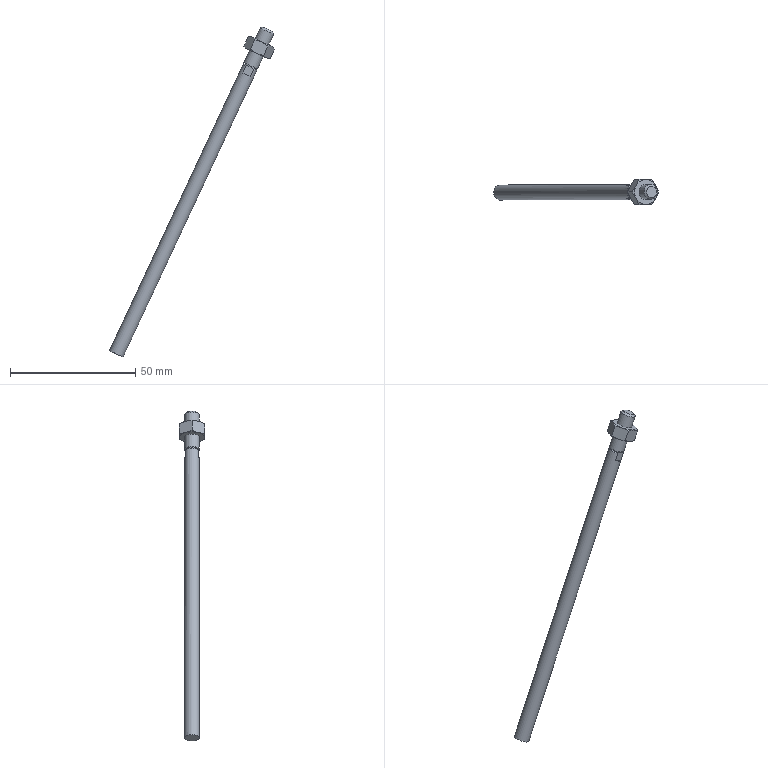Part | STEP file | 冲床-300配套压波_id674_x_t | 1 solid | 36 faces | box 65.907 x 10 x 131.805 mm | volume 4315 mm3 | plane 17 | cone 15 | cylinder 4 | commonest cylinder face diameters 6 x3 5 x1
STEP:
#1=CARTESIAN_POINT('',(2039.756,5.,-415.059));
#2=VERTEX_POINT('',#1);
#3=CARTESIAN_POINT('',(2036.951,5.,-414.243));
#4=VERTEX_POINT('',#3);
#5=CARTESIAN_POINT('',(2039.756,5.,-415.059));
#6=CARTESIAN_POINT('',(2038.786,5.,-414.907));
#7=CARTESIAN_POINT('',(2037.844,5.,-414.66));
#8=CARTESIAN_POINT('',(2036.951,5.,-414.243));
#9=B_SPLINE_CURVE_WITH_KNOTS('',3,(#5,#6,#7,#8),.UNSPECIFIED.,.F.,.F.,(4,4),(0.,1.),.UNSPECIFIED.);
#10=EDGE_CURVE('',#2,#4,#9,.T.);
#11=ORIENTED_EDGE('',*,*,#10,.T.);
#12=CARTESIAN_POINT('',(2034.524,5.,-412.618));
#13=VERTEX_POINT('',#12);
#14=CARTESIAN_POINT('',(2036.951,5.,-414.243));
#15=CARTESIAN_POINT('',(2036.058,5.,-413.827));
#16=CARTESIAN_POINT('',(2035.263,5.,-413.264));
#17=CARTESIAN_POINT('',(2034.524,5.,-412.618));
#18=B_SPLINE_CURVE_WITH_KNOTS('',3,(#14,#15,#16,#17),.UNSPECIFIED.,.F.,.F.,(4,4),(0.,1.),.UNSPECIFIED.);
#19=EDGE_CURVE('',#4,#13,#18,.T.);
#20=ORIENTED_EDGE('',*,*,#19,.T.);
#21=CARTESIAN_POINT('',(2036.261,5.,-408.896));
#22=VERTEX_POINT('',#21);
#23=CARTESIAN_POINT('',(2034.335,5.,-413.023));
#24=DIRECTION('',(0.4229,0.,0.9062));
#25=VECTOR('',#24,1.);
#26=LINE('',#23,#25);
#27=EDGE_CURVE('',#13,#22,#26,.T.);
#28=ORIENTED_EDGE('',*,*,#27,.T.);
#29=CARTESIAN_POINT('',(2039.065,5.,-409.712));
#30=VERTEX_POINT('',#29);
#31=CARTESIAN_POINT('',(2036.261,5.,-408.896));
#32=CARTESIAN_POINT('',(2037.23,5.,-409.049));
#33=CARTESIAN_POINT('',(2038.173,5.,-409.296));
#34=CARTESIAN_POINT('',(2039.065,5.,-409.712));
#35=B_SPLINE_CURVE_WITH_KNOTS('',3,(#31,#32,#33,#34),.UNSPECIFIED.,.F.,.F.,(4,4),(0.,1.),.UNSPECIFIED.);
#36=EDGE_CURVE('',#22,#30,#35,.T.);
#37=ORIENTED_EDGE('',*,*,#36,.T.);
#38=CARTESIAN_POINT('',(2041.493,5.,-411.338));
#39=VERTEX_POINT('',#38);
#40=CARTESIAN_POINT('',(2039.065,5.,-409.712));
#41=CARTESIAN_POINT('',(2039.958,5.,-410.129));
#42=CARTESIAN_POINT('',(2040.753,5.,-410.692));
#43=CARTESIAN_POINT('',(2041.493,5.,-411.338));
#44=B_SPLINE_CURVE_WITH_KNOTS('',3,(#40,#41,#42,#43),.UNSPECIFIED.,.F.,.F.,(4,4),(0.,1.),.UNSPECIFIED.);
#45=EDGE_CURVE('',#30,#39,#44,.T.);
#46=ORIENTED_EDGE('',*,*,#45,.T.);
#47=CARTESIAN_POINT('',(2039.567,5.,-415.464));
#48=DIRECTION('',(0.4229,0.,0.9062));
#49=VECTOR('',#48,1.);
#50=LINE('',#47,#49);
#51=EDGE_CURVE('',#2,#39,#50,.T.);
#52=ORIENTED_EDGE('',*,*,#51,.F.);
#53=EDGE_LOOP('',(#11,#20,#28,#37,#46,#52));
#54=FACE_OUTER_BOUND('',#53,.T.);
#55=CARTESIAN_POINT('',(2039.567,5.,-415.464));
#56=DIRECTION('',(0.,1.,0.));
#57=DIRECTION('',(0.9062,0.,-0.4229));
#58=AXIS2_PLACEMENT_3D('',#55,#56,#57);
#59=PLANE('',#58);
#60=ADVANCED_FACE('',(#54),#59,.T.);
#61=CARTESIAN_POINT('',(2042.372,0.,-416.28));
#62=VERTEX_POINT('',#61);
#63=CARTESIAN_POINT('',(2040.875,2.5,-416.074));
#64=VERTEX_POINT('',#63);
#65=CARTESIAN_POINT('',(2042.372,0.,-416.28));
#66=CARTESIAN_POINT('',(2041.829,0.8168,-416.327));
#67=CARTESIAN_POINT('',(2041.321,1.647,-416.283));
#68=CARTESIAN_POINT('',(2040.875,2.5,-416.074));
#69=B_SPLINE_CURVE_WITH_KNOTS('',3,(#65,#66,#67,#68),.UNSPECIFIED.,.F.,.F.,(4,4),(0.,1.),.UNSPECIFIED.);
#70=EDGE_CURVE('',#62,#64,#69,.T.);
#71=ORIENTED_EDGE('',*,*,#70,.T.);
#72=CARTESIAN_POINT('',(2040.875,2.5,-416.074));
#73=CARTESIAN_POINT('',(2040.429,3.353,-415.866));
#74=CARTESIAN_POINT('',(2040.068,4.183,-415.506));
#75=CARTESIAN_POINT('',(2039.756,5.,-415.059));
#76=B_SPLINE_CURVE_WITH_KNOTS('',3,(#72,#73,#74,#75),.UNSPECIFIED.,.F.,.F.,(4,4),(0.,1.),.UNSPECIFIED.);
#77=EDGE_CURVE('',#64,#2,#76,.T.);
#78=ORIENTED_EDGE('',*,*,#77,.T.);
#79=ORIENTED_EDGE('',*,*,#51,.T.);
#80=CARTESIAN_POINT('',(2042.989,2.5,-411.544));
#81=VERTEX_POINT('',#80);
#82=CARTESIAN_POINT('',(2041.493,5.,-411.338));
#83=CARTESIAN_POINT('',(2042.035,4.183,-411.291));
#84=CARTESIAN_POINT('',(2042.543,3.353,-411.335));
#85=CARTESIAN_POINT('',(2042.989,2.5,-411.544));
#86=B_SPLINE_CURVE_WITH_KNOTS('',3,(#82,#83,#84,#85),.UNSPECIFIED.,.F.,.F.,(4,4),(0.,1.),.UNSPECIFIED.);
#87=EDGE_CURVE('',#39,#81,#86,.T.);
#88=ORIENTED_EDGE('',*,*,#87,.T.);
#89=CARTESIAN_POINT('',(2044.108,0.,-412.559));
#90=VERTEX_POINT('',#89);
#91=CARTESIAN_POINT('',(2042.989,2.5,-411.544));
#92=CARTESIAN_POINT('',(2043.436,1.647,-411.752));
#93=CARTESIAN_POINT('',(2043.796,0.8168,-412.112));
#94=CARTESIAN_POINT('',(2044.108,0.,-412.559));
#95=B_SPLINE_CURVE_WITH_KNOTS('',3,(#91,#92,#93,#94),.UNSPECIFIED.,.F.,.F.,(4,4),(0.,1.),.UNSPECIFIED.);
#96=EDGE_CURVE('',#81,#90,#95,.T.);
#97=ORIENTED_EDGE('',*,*,#96,.T.);
#98=CARTESIAN_POINT('',(2042.183,0.,-416.685));
#99=DIRECTION('',(0.4229,0.,0.9062));
#100=VECTOR('',#99,1.);
#101=LINE('',#98,#100);
#102=EDGE_CURVE('',#62,#90,#101,.T.);
#103=ORIENTED_EDGE('',*,*,#102,.F.);
#104=EDGE_LOOP('',(#71,#78,#79,#88,#97,#103));
#105=FACE_OUTER_BOUND('',#104,.T.);
#106=CARTESIAN_POINT('',(2042.183,0.,-416.685));
#107=DIRECTION('',(0.7848,0.5,-0.3662));
#108=DIRECTION('',(0.4531,-0.866,-0.2114));
#109=AXIS2_PLACEMENT_3D('',#106,#107,#108);
#110=PLANE('',#109);
#111=ADVANCED_FACE('',(#105),#110,.T.);
#112=ORIENTED_EDGE('',*,*,#10,.F.);
#113=ORIENTED_EDGE('',*,*,#77,.F.);
#114=CARTESIAN_POINT('',(2036.951,0.,-414.243));
#115=DIRECTION('',(0.4229,0.,0.9062));
#116=DIRECTION('',(0.,-1.,0.));
#117=AXIS2_PLACEMENT_3D('',#114,#115,#116);
#118=CIRCLE('',#117,5.);
#119=EDGE_CURVE('',#64,#4,#118,.T.);
#120=ORIENTED_EDGE('',*,*,#119,.T.);
#121=EDGE_LOOP('',(#112,#113,#120));
#122=FACE_OUTER_BOUND('',#121,.T.);
#123=CARTESIAN_POINT('',(2036.951,0.,-414.243));
#124=DIRECTION('',(0.4229,0.,0.9062));
#125=DIRECTION('',(0.,1.,0.));
#126=AXIS2_PLACEMENT_3D('',#123,#124,#125);
#127=CONICAL_SURFACE('',#126,5.,60.);
#128=ADVANCED_FACE('',(#122),#127,.T.);
#129=ORIENTED_EDGE('',*,*,#45,.F.);
#130=CARTESIAN_POINT('',(2039.065,0.,-409.712));
#131=DIRECTION('',(0.4229,0.,0.9062));
#132=DIRECTION('',(0.,-1.,0.));
#133=AXIS2_PLACEMENT_3D('',#130,#131,#132);
#134=CIRCLE('',#133,5.);
#135=EDGE_CURVE('',#81,#30,#134,.T.);
#136=ORIENTED_EDGE('',*,*,#135,.F.);
#137=ORIENTED_EDGE('',*,*,#87,.F.);
#138=EDGE_LOOP('',(#129,#136,#137));
#139=FACE_OUTER_BOUND('',#138,.T.);
#140=CARTESIAN_POINT('',(2038.877,0.,-410.117));
#141=DIRECTION('',(-0.4229,0.,-0.9062));
#142=DIRECTION('',(0.,-1.,0.));
#143=AXIS2_PLACEMENT_3D('',#140,#141,#142);
#144=CONICAL_SURFACE('',#143,5.774,60.);
#145=ADVANCED_FACE('',(#139),#144,.T.);
#146=CARTESIAN_POINT('',(2033.027,2.5,-412.412));
#147=VERTEX_POINT('',#146);
#148=CARTESIAN_POINT('',(2034.524,5.,-412.618));
#149=CARTESIAN_POINT('',(2033.981,4.183,-412.665));
#150=CARTESIAN_POINT('',(2033.474,3.353,-412.621));
#151=CARTESIAN_POINT('',(2033.027,2.5,-412.412));
#152=B_SPLINE_CURVE_WITH_KNOTS('',3,(#148,#149,#150,#151),.UNSPECIFIED.,.F.,.F.,(4,4),(0.,1.),.UNSPECIFIED.);
#153=EDGE_CURVE('',#13,#147,#152,.T.);
#154=ORIENTED_EDGE('',*,*,#153,.F.);
#155=ORIENTED_EDGE('',*,*,#19,.F.);
#156=CARTESIAN_POINT('',(2036.951,0.,-414.243));
#157=DIRECTION('',(0.4229,0.,0.9062));
#158=DIRECTION('',(0.,-1.,0.));
#159=AXIS2_PLACEMENT_3D('',#156,#157,#158);
#160=CIRCLE('',#159,5.);
#161=EDGE_CURVE('',#4,#147,#160,.T.);
#162=ORIENTED_EDGE('',*,*,#161,.T.);
#163=EDGE_LOOP('',(#154,#155,#162));
#164=FACE_OUTER_BOUND('',#163,.T.);
#165=CARTESIAN_POINT('',(2036.951,0.,-414.243));
#166=DIRECTION('',(0.4229,0.,0.9062));
#167=DIRECTION('',(0.,1.,0.));
#168=AXIS2_PLACEMENT_3D('',#165,#166,#167);
#169=CONICAL_SURFACE('',#168,5.,60.);
#170=ADVANCED_FACE('',(#164),#169,.T.);
#171=CARTESIAN_POINT('',(2035.141,2.5,-407.881));
#172=VERTEX_POINT('',#171);
#173=CARTESIAN_POINT('',(2035.141,2.5,-407.881));
#174=CARTESIAN_POINT('',(2035.588,3.353,-408.09));
#175=CARTESIAN_POINT('',(2035.948,4.183,-408.45));
#176=CARTESIAN_POINT('',(2036.261,5.,-408.896));
#177=B_SPLINE_CURVE_WITH_KNOTS('',3,(#173,#174,#175,#176),.UNSPECIFIED.,.F.,.F.,(4,4),(0.,1.),.UNSPECIFIED.);
#178=EDGE_CURVE('',#172,#22,#177,.T.);
#179=ORIENTED_EDGE('',*,*,#178,.F.);
#180=CARTESIAN_POINT('',(2039.065,0.,-409.712));
#181=DIRECTION('',(0.4229,0.,0.9062));
#182=DIRECTION('',(0.,-1.,0.));
#183=AXIS2_PLACEMENT_3D('',#180,#181,#182);
#184=CIRCLE('',#183,5.);
#185=EDGE_CURVE('',#30,#172,#184,.T.);
#186=ORIENTED_EDGE('',*,*,#185,.F.);
#187=ORIENTED_EDGE('',*,*,#36,.F.);
#188=EDGE_LOOP('',(#179,#186,#187));
#189=FACE_OUTER_BOUND('',#188,.T.);
#190=CARTESIAN_POINT('',(2038.877,0.,-410.117));
#191=DIRECTION('',(-0.4229,0.,-0.9062));
#192=DIRECTION('',(0.,-1.,0.));
#193=AXIS2_PLACEMENT_3D('',#190,#191,#192);
#194=CONICAL_SURFACE('',#193,5.774,60.);
#195=ADVANCED_FACE('',(#189),#194,.T.);
#196=ORIENTED_EDGE('',*,*,#153,.T.);
#197=CARTESIAN_POINT('',(2031.908,0.,-411.397));
#198=VERTEX_POINT('',#197);
#199=CARTESIAN_POINT('',(2033.027,2.5,-412.412));
#200=CARTESIAN_POINT('',(2032.581,1.647,-412.204));
#201=CARTESIAN_POINT('',(2032.22,0.8168,-411.843));
#202=CARTESIAN_POINT('',(2031.908,0.,-411.397));
#203=B_SPLINE_CURVE_WITH_KNOTS('',3,(#199,#200,#201,#202),.UNSPECIFIED.,.F.,.F.,(4,4),(0.,1.),.UNSPECIFIED.);
#204=EDGE_CURVE('',#147,#198,#203,.T.);
#205=ORIENTED_EDGE('',*,*,#204,.T.);
#206=CARTESIAN_POINT('',(2033.645,0.,-407.676));
#207=VERTEX_POINT('',#206);
#208=CARTESIAN_POINT('',(2031.719,0.,-411.802));
#209=DIRECTION('',(0.4229,0.,0.9062));
#210=VECTOR('',#209,1.);
#211=LINE('',#208,#210);
#212=EDGE_CURVE('',#198,#207,#211,.T.);
#213=ORIENTED_EDGE('',*,*,#212,.T.);
#214=CARTESIAN_POINT('',(2033.645,0.,-407.676));
#215=CARTESIAN_POINT('',(2034.187,0.8168,-407.628));
#216=CARTESIAN_POINT('',(2034.695,1.647,-407.673));
#217=CARTESIAN_POINT('',(2035.141,2.5,-407.881));
#218=B_SPLINE_CURVE_WITH_KNOTS('',3,(#214,#215,#216,#217),.UNSPECIFIED.,.F.,.F.,(4,4),(0.,1.),.UNSPECIFIED.);
#219=EDGE_CURVE('',#207,#172,#218,.T.);
#220=ORIENTED_EDGE('',*,*,#219,.T.);
#221=ORIENTED_EDGE('',*,*,#178,.T.);
#222=ORIENTED_EDGE('',*,*,#27,.F.);
#223=EDGE_LOOP('',(#196,#205,#213,#220,#221,#222));
#224=FACE_OUTER_BOUND('',#223,.T.);
#225=CARTESIAN_POINT('',(2034.335,5.,-413.023));
#226=DIRECTION('',(-0.7848,0.5,0.3662));
#227=DIRECTION('',(0.4531,0.866,-0.2114));
#228=AXIS2_PLACEMENT_3D('',#225,#226,#227);
#229=PLANE('',#228);
#230=ADVANCED_FACE('',(#224),#229,.T.);
#231=CARTESIAN_POINT('',(2039.756,-5.,-415.059));
#232=VERTEX_POINT('',#231);
#233=CARTESIAN_POINT('',(2040.875,-2.5,-416.074));
#234=VERTEX_POINT('',#233);
#235=CARTESIAN_POINT('',(2039.756,-5.,-415.059));
#236=CARTESIAN_POINT('',(2040.068,-4.183,-415.506));
#237=CARTESIAN_POINT('',(2040.429,-3.353,-415.866));
#238=CARTESIAN_POINT('',(2040.875,-2.5,-416.074));
#239=B_SPLINE_CURVE_WITH_KNOTS('',3,(#235,#236,#237,#238),.UNSPECIFIED.,.F.,.F.,(4,4),(0.,1.),.UNSPECIFIED.);
#240=EDGE_CURVE('',#232,#234,#239,.T.);
#241=ORIENTED_EDGE('',*,*,#240,.T.);
#242=CARTESIAN_POINT('',(2040.875,-2.5,-416.074));
#243=CARTESIAN_POINT('',(2041.321,-1.647,-416.283));
#244=CARTESIAN_POINT('',(2041.829,-0.8168,-416.327));
#245=CARTESIAN_POINT('',(2042.372,0.,-416.28));
#246=B_SPLINE_CURVE_WITH_KNOTS('',3,(#242,#243,#244,#245),.UNSPECIFIED.,.F.,.F.,(4,4),(0.,1.),.UNSPECIFIED.);
#247=EDGE_CURVE('',#234,#62,#246,.T.);
#248=ORIENTED_EDGE('',*,*,#247,.T.);
#249=ORIENTED_EDGE('',*,*,#102,.T.);
#250=CARTESIAN_POINT('',(2042.989,-2.5,-411.544));
#251=VERTEX_POINT('',#250);
#252=CARTESIAN_POINT('',(2044.108,0.,-412.559));
#253=CARTESIAN_POINT('',(2043.796,-0.8168,-412.112));
#254=CARTESIAN_POINT('',(2043.436,-1.647,-411.752));
#255=CARTESIAN_POINT('',(2042.989,-2.5,-411.544));
#256=B_SPLINE_CURVE_WITH_KNOTS('',3,(#252,#253,#254,#255),.UNSPECIFIED.,.F.,.F.,(4,4),(0.,1.),.UNSPECIFIED.);
#257=EDGE_CURVE('',#90,#251,#256,.T.);
#258=ORIENTED_EDGE('',*,*,#257,.T.);
#259=CARTESIAN_POINT('',(2041.493,-5.,-411.338));
#260=VERTEX_POINT('',#259);
#261=CARTESIAN_POINT('',(2042.989,-2.5,-411.544));
#262=CARTESIAN_POINT('',(2042.543,-3.353,-411.335));
#263=CARTESIAN_POINT('',(2042.035,-4.183,-411.291));
#264=CARTESIAN_POINT('',(2041.493,-5.,-411.338));
#265=B_SPLINE_CURVE_WITH_KNOTS('',3,(#261,#262,#263,#264),.UNSPECIFIED.,.F.,.F.,(4,4),(0.,1.),.UNSPECIFIED.);
#266=EDGE_CURVE('',#251,#260,#265,.T.);
#267=ORIENTED_EDGE('',*,*,#266,.T.);
#268=CARTESIAN_POINT('',(2039.567,-5.,-415.464));
#269=DIRECTION('',(0.4229,0.,0.9062));
#270=VECTOR('',#269,1.);
#271=LINE('',#268,#270);
#272=EDGE_CURVE('',#232,#260,#271,.T.);
#273=ORIENTED_EDGE('',*,*,#272,.F.);
#274=EDGE_LOOP('',(#241,#248,#249,#258,#267,#273));
#275=FACE_OUTER_BOUND('',#274,.T.);
#276=CARTESIAN_POINT('',(2039.567,-5.,-415.464));
#277=DIRECTION('',(0.7848,-0.5,-0.3662));
#278=DIRECTION('',(-0.4531,-0.866,0.2114));
#279=AXIS2_PLACEMENT_3D('',#276,#277,#278);
#280=PLANE('',#279);
#281=ADVANCED_FACE('',(#275),#280,.T.);
#282=ORIENTED_EDGE('',*,*,#257,.F.);
#283=ORIENTED_EDGE('',*,*,#96,.F.);
#284=CARTESIAN_POINT('',(2039.065,0.,-409.712));
#285=DIRECTION('',(0.4229,0.,0.9062));
#286=DIRECTION('',(0.,-1.,0.));
#287=AXIS2_PLACEMENT_3D('',#284,#285,#286);
#288=CIRCLE('',#287,5.);
#289=EDGE_CURVE('',#251,#81,#288,.T.);
#290=ORIENTED_EDGE('',*,*,#289,.F.);
#291=EDGE_LOOP('',(#282,#283,#290));
#292=FACE_OUTER_BOUND('',#291,.T.);
#293=CARTESIAN_POINT('',(2038.877,0.,-410.117));
#294=DIRECTION('',(-0.4229,0.,-0.9062));
#295=DIRECTION('',(0.,-1.,0.));
#296=AXIS2_PLACEMENT_3D('',#293,#294,#295);
#297=CONICAL_SURFACE('',#296,5.774,60.);
#298=ADVANCED_FACE('',(#292),#297,.T.);
#299=ORIENTED_EDGE('',*,*,#247,.F.);
#300=CARTESIAN_POINT('',(2036.951,0.,-414.243));
#301=DIRECTION('',(0.4229,0.,0.9062));
#302=DIRECTION('',(0.,-1.,0.));
#303=AXIS2_PLACEMENT_3D('',#300,#301,#302);
#304=CIRCLE('',#303,5.);
#305=EDGE_CURVE('',#234,#64,#304,.T.);
#306=ORIENTED_EDGE('',*,*,#305,.T.);
#307=ORIENTED_EDGE('',*,*,#70,.F.);
#308=EDGE_LOOP('',(#299,#306,#307));
#309=FACE_OUTER_BOUND('',#308,.T.);
#310=CARTESIAN_POINT('',(2036.951,0.,-414.243));
#311=DIRECTION('',(0.4229,0.,0.9062));
#312=DIRECTION('',(0.,1.,0.));
#313=AXIS2_PLACEMENT_3D('',#310,#311,#312);
#314=CONICAL_SURFACE('',#313,5.,60.);
#315=ADVANCED_FACE('',(#309),#314,.T.);
#316=CARTESIAN_POINT('',(2036.951,-5.,-414.243));
#317=VERTEX_POINT('',#316);
#318=CARTESIAN_POINT('',(2036.951,0.,-414.243));
#319=DIRECTION('',(0.4229,0.,0.9062));
#320=DIRECTION('',(0.,-1.,0.));
#321=AXIS2_PLACEMENT_3D('',#318,#319,#320);
#322=CIRCLE('',#321,5.);
#323=EDGE_CURVE('',#317,#234,#322,.T.);
#324=ORIENTED_EDGE('',*,*,#323,.F.);
#325=CARTESIAN_POINT('',(2033.027,-2.5,-412.412));
#326=VERTEX_POINT('',#325);
#327=CARTESIAN_POINT('',(2036.951,0.,-414.243));
#328=DIRECTION('',(0.4229,0.,0.9062));
#329=DIRECTION('',(0.,-1.,0.));
#330=AXIS2_PLACEMENT_3D('',#327,#328,#329);
#331=CIRCLE('',#330,5.);
#332=EDGE_CURVE('',#326,#317,#331,.T.);
#333=ORIENTED_EDGE('',*,*,#332,.F.);
#334=CARTESIAN_POINT('',(2036.951,0.,-414.243));
#335=DIRECTION('',(0.4229,0.,0.9062));
#336=DIRECTION('',(0.,-1.,0.));
#337=AXIS2_PLACEMENT_3D('',#334,#335,#336);
#338=CIRCLE('',#337,5.);
#339=EDGE_CURVE('',#147,#326,#338,.T.);
#340=ORIENTED_EDGE('',*,*,#339,.F.);
#341=ORIENTED_EDGE('',*,*,#161,.F.);
#342=ORIENTED_EDGE('',*,*,#119,.F.);
#343=ORIENTED_EDGE('',*,*,#305,.F.);
#344=EDGE_LOOP('',(#324,#333,#340,#341,#342,#343));
#345=FACE_BOUND('',#344,.T.);
#346=CARTESIAN_POINT('',(2039.67,0.,-415.512));
#347=VERTEX_POINT('',#346);
#348=CARTESIAN_POINT('',(2036.951,0.,-414.243));
#349=DIRECTION('',(0.4229,0.,0.9062));
#350=DIRECTION('',(0.9062,0.,-0.4229));
#351=AXIS2_PLACEMENT_3D('',#348,#349,#350);
#352=CIRCLE('',#351,3.);
#353=EDGE_CURVE('',#347,#347,#352,.T.);
#354=ORIENTED_EDGE('',*,*,#353,.T.);
#355=EDGE_LOOP('',(#354));
#356=FACE_BOUND('',#355,.T.);
#357=CARTESIAN_POINT('',(2041.482,0.,-416.358));
#358=DIRECTION('',(0.4229,0.,0.9062));
#359=DIRECTION('',(0.,1.,0.));
#360=AXIS2_PLACEMENT_3D('',#357,#358,#359);
#361=PLANE('',#360);
#362=ADVANCED_FACE('',(#345,#356),#361,.F.);
#363=CARTESIAN_POINT('',(2036.347,0.,-408.444));
#364=VERTEX_POINT('',#363);
#365=CARTESIAN_POINT('',(2039.065,0.,-409.712));
#366=DIRECTION('',(0.4229,0.,0.9062));
#367=DIRECTION('',(-0.9062,0.,0.4229));
#368=AXIS2_PLACEMENT_3D('',#365,#366,#367);
#369=CIRCLE('',#368,3.);
#370=EDGE_CURVE('',#364,#364,#369,.T.);
#371=ORIENTED_EDGE('',*,*,#370,.F.);
#372=EDGE_LOOP('',(#371));
#373=FACE_BOUND('',#372,.T.);
#374=CARTESIAN_POINT('',(2039.065,-5.,-409.712));
#375=VERTEX_POINT('',#374);
#376=CARTESIAN_POINT('',(2039.065,0.,-409.712));
#377=DIRECTION('',(0.4229,0.,0.9062));
#378=DIRECTION('',(0.,-1.,0.));
#379=AXIS2_PLACEMENT_3D('',#376,#377,#378);
#380=CIRCLE('',#379,5.);
#381=EDGE_CURVE('',#375,#251,#380,.T.);
#382=ORIENTED_EDGE('',*,*,#381,.T.);
#383=ORIENTED_EDGE('',*,*,#289,.T.);
#384=ORIENTED_EDGE('',*,*,#135,.T.);
#385=ORIENTED_EDGE('',*,*,#185,.T.);
#386=CARTESIAN_POINT('',(2035.141,-2.5,-407.881));
#387=VERTEX_POINT('',#386);
#388=CARTESIAN_POINT('',(2039.065,0.,-409.712));
#389=DIRECTION('',(0.4229,0.,0.9062));
#390=DIRECTION('',(0.,-1.,0.));
#391=AXIS2_PLACEMENT_3D('',#388,#389,#390);
#392=CIRCLE('',#391,5.);
#393=EDGE_CURVE('',#172,#387,#392,.T.);
#394=ORIENTED_EDGE('',*,*,#393,.T.);
#395=CARTESIAN_POINT('',(2039.065,0.,-409.712));
#396=DIRECTION('',(0.4229,0.,0.9062));
#397=DIRECTION('',(0.,-1.,0.));
#398=AXIS2_PLACEMENT_3D('',#395,#396,#397);
#399=CIRCLE('',#398,5.);
#400=EDGE_CURVE('',#387,#375,#399,.T.);
#401=ORIENTED_EDGE('',*,*,#400,.T.);
#402=EDGE_LOOP('',(#382,#383,#384,#385,#394,#401));
#403=FACE_BOUND('',#402,.T.);
#404=CARTESIAN_POINT('',(2043.596,0.,-411.827));
#405=DIRECTION('',(-0.4229,0.,-0.9062));
#406=DIRECTION('',(0.,-1.,0.));
#407=AXIS2_PLACEMENT_3D('',#404,#405,#406);
#408=PLANE('',#407);
#409=ADVANCED_FACE('',(#373,#403),#408,.F.);
#410=CARTESIAN_POINT('',(2031.908,0.,-411.397));
#411=CARTESIAN_POINT('',(2032.22,-0.8168,-411.843));
#412=CARTESIAN_POINT('',(2032.581,-1.647,-412.204));
#413=CARTESIAN_POINT('',(2033.027,-2.5,-412.412));
#414=B_SPLINE_CURVE_WITH_KNOTS('',3,(#410,#411,#412,#413),.UNSPECIFIED.,.F.,.F.,(4,4),(0.,1.),.UNSPECIFIED.);
#415=EDGE_CURVE('',#198,#326,#414,.T.);
#416=ORIENTED_EDGE('',*,*,#415,.T.);
#417=CARTESIAN_POINT('',(2034.524,-5.,-412.618));
#418=VERTEX_POINT('',#417);
#419=CARTESIAN_POINT('',(2033.027,-2.5,-412.412));
#420=CARTESIAN_POINT('',(2033.474,-3.353,-412.621));
#421=CARTESIAN_POINT('',(2033.981,-4.183,-412.665));
#422=CARTESIAN_POINT('',(2034.524,-5.,-412.618));
#423=B_SPLINE_CURVE_WITH_KNOTS('',3,(#419,#420,#421,#422),.UNSPECIFIED.,.F.,.F.,(4,4),(0.,1.),.UNSPECIFIED.);
#424=EDGE_CURVE('',#326,#418,#423,.T.);
#425=ORIENTED_EDGE('',*,*,#424,.T.);
#426=CARTESIAN_POINT('',(2036.261,-5.,-408.896));
#427=VERTEX_POINT('',#426);
#428=CARTESIAN_POINT('',(2034.335,-5.,-413.023));
#429=DIRECTION('',(0.4229,0.,0.9062));
#430=VECTOR('',#429,1.);
#431=LINE('',#428,#430);
#432=EDGE_CURVE('',#418,#427,#431,.T.);
#433=ORIENTED_EDGE('',*,*,#432,.T.);
#434=CARTESIAN_POINT('',(2036.261,-5.,-408.896));
#435=CARTESIAN_POINT('',(2035.948,-4.183,-408.45));
#436=CARTESIAN_POINT('',(2035.588,-3.353,-408.09));
#437=CARTESIAN_POINT('',(2035.141,-2.5,-407.881));
#438=B_SPLINE_CURVE_WITH_KNOTS('',3,(#434,#435,#436,#437),.UNSPECIFIED.,.F.,.F.,(4,4),(0.,1.),.UNSPECIFIED.);
#439=EDGE_CURVE('',#427,#387,#438,.T.);
#440=ORIENTED_EDGE('',*,*,#439,.T.);
#441=CARTESIAN_POINT('',(2035.141,-2.5,-407.881));
#442=CARTESIAN_POINT('',(2034.695,-1.647,-407.673));
#443=CARTESIAN_POINT('',(2034.187,-0.8168,-407.628));
#444=CARTESIAN_POINT('',(2033.645,0.,-407.676));
#445=B_SPLINE_CURVE_WITH_KNOTS('',3,(#441,#442,#443,#444),.UNSPECIFIED.,.F.,.F.,(4,4),(0.,1.),.UNSPECIFIED.);
#446=EDGE_CURVE('',#387,#207,#445,.T.);
#447=ORIENTED_EDGE('',*,*,#446,.T.);
#448=ORIENTED_EDGE('',*,*,#212,.F.);
#449=EDGE_LOOP('',(#416,#425,#433,#440,#447,#448));
#450=FACE_OUTER_BOUND('',#449,.T.);
#451=CARTESIAN_POINT('',(2031.719,0.,-411.802));
#452=DIRECTION('',(-0.7848,-0.5,0.3662));
#453=DIRECTION('',(-0.4531,0.866,0.2114));
#454=AXIS2_PLACEMENT_3D('',#451,#452,#453);
#455=PLANE('',#454);
#456=ADVANCED_FACE('',(#450),#455,.T.);
#457=ORIENTED_EDGE('',*,*,#415,.F.);
#458=ORIENTED_EDGE('',*,*,#204,.F.);
#459=ORIENTED_EDGE('',*,*,#339,.T.);
#460=EDGE_LOOP('',(#457,#458,#459));
#461=FACE_OUTER_BOUND('',#460,.T.);
#462=CARTESIAN_POINT('',(2036.951,0.,-414.243));
#463=DIRECTION('',(0.4229,0.,0.9062));
#464=DIRECTION('',(0.,1.,0.));
#465=AXIS2_PLACEMENT_3D('',#462,#463,#464);
#466=CONICAL_SURFACE('',#465,5.,60.);
#467=ADVANCED_FACE('',(#461),#466,.T.);
#468=ORIENTED_EDGE('',*,*,#446,.F.);
#469=ORIENTED_EDGE('',*,*,#393,.F.);
#470=ORIENTED_EDGE('',*,*,#219,.F.);
#471=EDGE_LOOP('',(#468,#469,#470));
#472=FACE_OUTER_BOUND('',#471,.T.);
#473=CARTESIAN_POINT('',(2038.877,0.,-410.117));
#474=DIRECTION('',(-0.4229,0.,-0.9062));
#475=DIRECTION('',(0.,-1.,0.));
#476=AXIS2_PLACEMENT_3D('',#473,#474,#475);
#477=CONICAL_SURFACE('',#476,5.774,60.);
#478=ADVANCED_FACE('',(#472),#477,.T.);
#479=ORIENTED_EDGE('',*,*,#266,.F.);
#480=ORIENTED_EDGE('',*,*,#381,.F.);
#481=CARTESIAN_POINT('',(2041.493,-5.,-411.338));
#482=CARTESIAN_POINT('',(2040.753,-5.,-410.692));
#483=CARTESIAN_POINT('',(2039.958,-5.,-410.129));
#484=CARTESIAN_POINT('',(2039.065,-5.,-409.712));
#485=B_SPLINE_CURVE_WITH_KNOTS('',3,(#481,#482,#483,#484),.UNSPECIFIED.,.F.,.F.,(4,4),(0.,1.),.UNSPECIFIED.);
#486=EDGE_CURVE('',#260,#375,#485,.T.);
#487=ORIENTED_EDGE('',*,*,#486,.F.);
#488=EDGE_LOOP('',(#479,#480,#487));
#489=FACE_OUTER_BOUND('',#488,.T.);
#490=CARTESIAN_POINT('',(2038.877,0.,-410.117));
#491=DIRECTION('',(-0.4229,0.,-0.9062));
#492=DIRECTION('',(0.,-1.,0.));
#493=AXIS2_PLACEMENT_3D('',#490,#491,#492);
#494=CONICAL_SURFACE('',#493,5.774,60.);
#495=ADVANCED_FACE('',(#489),#494,.T.);
#496=CARTESIAN_POINT('',(2036.951,-5.,-414.243));
#497=CARTESIAN_POINT('',(2037.844,-5.,-414.66));
#498=CARTESIAN_POINT('',(2038.786,-5.,-414.907));
#499=CARTESIAN_POINT('',(2039.756,-5.,-415.059));
#500=B_SPLINE_CURVE_WITH_KNOTS('',3,(#496,#497,#498,#499),.UNSPECIFIED.,.F.,.F.,(4,4),(0.,1.),.UNSPECIFIED.);
#501=EDGE_CURVE('',#317,#232,#500,.T.);
#502=ORIENTED_EDGE('',*,*,#501,.F.);
#503=ORIENTED_EDGE('',*,*,#323,.T.);
#504=ORIENTED_EDGE('',*,*,#240,.F.);
#505=EDGE_LOOP('',(#502,#503,#504));
#506=FACE_OUTER_BOUND('',#505,.T.);
#507=CARTESIAN_POINT('',(2036.951,0.,-414.243));
#508=DIRECTION('',(0.4229,0.,0.9062));
#509=DIRECTION('',(0.,1.,0.));
#510=AXIS2_PLACEMENT_3D('',#507,#508,#509);
#511=CONICAL_SURFACE('',#510,5.,60.);
#512=ADVANCED_FACE('',(#506),#511,.T.);
#513=CARTESIAN_POINT('',(2034.524,-5.,-412.618));
#514=CARTESIAN_POINT('',(2035.263,-5.,-413.264));
#515=CARTESIAN_POINT('',(2036.058,-5.,-413.827));
#516=CARTESIAN_POINT('',(2036.951,-5.,-414.243));
#517=B_SPLINE_CURVE_WITH_KNOTS('',3,(#513,#514,#515,#516),.UNSPECIFIED.,.F.,.F.,(4,4),(0.,1.),.UNSPECIFIED.);
#518=EDGE_CURVE('',#418,#317,#517,.T.);
#519=ORIENTED_EDGE('',*,*,#518,.T.);
#520=ORIENTED_EDGE('',*,*,#501,.T.);
#521=ORIENTED_EDGE('',*,*,#272,.T.);
#522=ORIENTED_EDGE('',*,*,#486,.T.);
#523=CARTESIAN_POINT('',(2039.065,-5.,-409.712));
#524=CARTESIAN_POINT('',(2038.173,-5.,-409.296));
#525=CARTESIAN_POINT('',(2037.23,-5.,-409.049));
#526=CARTESIAN_POINT('',(2036.261,-5.,-408.896));
#527=B_SPLINE_CURVE_WITH_KNOTS('',3,(#523,#524,#525,#526),.UNSPECIFIED.,.F.,.F.,(4,4),(0.,1.),.UNSPECIFIED.);
#528=EDGE_CURVE('',#375,#427,#527,.T.);
#529=ORIENTED_EDGE('',*,*,#528,.T.);
#530=ORIENTED_EDGE('',*,*,#432,.F.);
#531=EDGE_LOOP('',(#519,#520,#521,#522,#529,#530));
#532=FACE_OUTER_BOUND('',#531,.T.);
#533=CARTESIAN_POINT('',(2034.335,-5.,-413.023));
#534=DIRECTION('',(0.,-1.,0.));
#535=DIRECTION('',(-0.9062,0.,0.4229));
#536=AXIS2_PLACEMENT_3D('',#533,#534,#535);
#537=PLANE('',#536);
#538=ADVANCED_FACE('',(#532),#537,.T.);
#539=CARTESIAN_POINT('',(2031.907,0.,-417.959));
#540=VERTEX_POINT('',#539);
#541=CARTESIAN_POINT('',(2034.625,0.,-419.227));
#542=DIRECTION('',(-0.4229,0.,-0.9062));
#543=DIRECTION('',(-0.9062,0.,0.4229));
#544=AXIS2_PLACEMENT_3D('',#541,#542,#543);
#545=CIRCLE('',#544,3.);
#546=EDGE_CURVE('',#540,#540,#545,.T.);
#547=ORIENTED_EDGE('',*,*,#546,.F.);
#548=EDGE_LOOP('',(#547));
#549=FACE_BOUND('',#548,.T.);
#550=ORIENTED_EDGE('',*,*,#353,.F.);
#551=EDGE_LOOP('',(#550));
#552=FACE_BOUND('',#551,.T.);
#553=CARTESIAN_POINT('',(1980.92,0.,-534.313));
#554=DIRECTION('',(-0.4229,0.,-0.9062));
#555=DIRECTION('',(0.,-1.,0.));
#556=AXIS2_PLACEMENT_3D('',#553,#554,#555);
#557=CYLINDRICAL_SURFACE('',#556,3.);
#558=ADVANCED_FACE('',(#549,#552),#557,.T.);
#559=ORIENTED_EDGE('',*,*,#424,.F.);
#560=ORIENTED_EDGE('',*,*,#332,.T.);
#561=ORIENTED_EDGE('',*,*,#518,.F.);
#562=EDGE_LOOP('',(#559,#560,#561));
#563=FACE_OUTER_BOUND('',#562,.T.);
#564=CARTESIAN_POINT('',(2036.951,0.,-414.243));
#565=DIRECTION('',(0.4229,0.,0.9062));
#566=DIRECTION('',(0.,1.,0.));
#567=AXIS2_PLACEMENT_3D('',#564,#565,#566);
#568=CONICAL_SURFACE('',#567,5.,60.);
#569=ADVANCED_FACE('',(#563),#568,.T.);
#570=CARTESIAN_POINT('',(2038.355,0.,-404.139));
#571=VERTEX_POINT('',#570);
#572=CARTESIAN_POINT('',(2041.074,0.,-405.408));
#573=DIRECTION('',(-0.4229,0.,-0.9062));
#574=DIRECTION('',(-0.9062,0.,0.4229));
#575=AXIS2_PLACEMENT_3D('',#572,#573,#574);
#576=CIRCLE('',#575,3.);
#577=EDGE_CURVE('',#571,#571,#576,.T.);
#578=ORIENTED_EDGE('',*,*,#577,.T.);
#579=EDGE_LOOP('',(#578));
#580=FACE_BOUND('',#579,.T.);
#581=ORIENTED_EDGE('',*,*,#370,.T.);
#582=EDGE_LOOP('',(#581));
#583=FACE_BOUND('',#582,.T.);
#584=CARTESIAN_POINT('',(1980.92,0.,-534.313));
#585=DIRECTION('',(-0.4229,0.,-0.9062));
#586=DIRECTION('',(0.,-1.,0.));
#587=AXIS2_PLACEMENT_3D('',#584,#585,#586);
#588=CYLINDRICAL_SURFACE('',#587,3.);
#589=ADVANCED_FACE('',(#580,#583),#588,.T.);
#590=ORIENTED_EDGE('',*,*,#528,.F.);
#591=ORIENTED_EDGE('',*,*,#400,.F.);
#592=ORIENTED_EDGE('',*,*,#439,.F.);
#593=EDGE_LOOP('',(#590,#591,#592));
#594=FACE_OUTER_BOUND('',#593,.T.);
#595=CARTESIAN_POINT('',(2038.877,0.,-410.117));
#596=DIRECTION('',(-0.4229,0.,-0.9062));
#597=DIRECTION('',(0.,-1.,0.));
#598=AXIS2_PLACEMENT_3D('',#595,#596,#597);
#599=CONICAL_SURFACE('',#598,5.774,60.);
#600=ADVANCED_FACE('',(#594),#599,.T.);
#601=ORIENTED_EDGE('',*,*,#546,.T.);
#602=EDGE_LOOP('',(#601));
#603=FACE_BOUND('',#602,.T.);
#604=CARTESIAN_POINT('',(2034.625,2.5,-419.227));
#605=VERTEX_POINT('',#604);
#606=CARTESIAN_POINT('',(2034.625,0.,-419.227));
#607=DIRECTION('',(-0.4229,0.,-0.9062));
#608=DIRECTION('',(0.,1.,0.));
#609=AXIS2_PLACEMENT_3D('',#606,#607,#608);
#610=CIRCLE('',#609,2.5);
#611=EDGE_CURVE('',#605,#605,#610,.T.);
#612=ORIENTED_EDGE('',*,*,#611,.F.);
#613=EDGE_LOOP('',(#612));
#614=FACE_BOUND('',#613,.T.);
#615=CARTESIAN_POINT('',(2037.344,0.,-420.496));
#616=DIRECTION('',(-0.4229,0.,-0.9062));
#617=DIRECTION('',(0.,-1.,0.));
#618=AXIS2_PLACEMENT_3D('',#615,#616,#617);
#619=PLANE('',#618);
#620=ADVANCED_FACE('',(#603,#614),#619,.T.);
#621=CARTESIAN_POINT('',(2041.391,2.25,-404.728));
#622=VERTEX_POINT('',#621);
#623=CARTESIAN_POINT('',(2041.391,0.,-404.728));
#624=DIRECTION('',(-0.4229,0.,-0.9062));
#625=DIRECTION('',(0.,1.,0.));
#626=AXIS2_PLACEMENT_3D('',#623,#624,#625);
#627=CIRCLE('',#626,2.25);
#628=EDGE_CURVE('',#622,#622,#627,.T.);
#629=ORIENTED_EDGE('',*,*,#628,.T.);
#630=EDGE_LOOP('',(#629));
#631=FACE_BOUND('',#630,.T.);
#632=ORIENTED_EDGE('',*,*,#577,.F.);
#633=EDGE_LOOP('',(#632));
#634=FACE_BOUND('',#633,.T.);
#635=CARTESIAN_POINT('',(2041.074,0.,-405.408));
#636=DIRECTION('',(-0.4229,0.,-0.9062));
#637=DIRECTION('',(0.,-1.,0.));
#638=AXIS2_PLACEMENT_3D('',#635,#636,#637);
#639=CONICAL_SURFACE('',#638,3.,45.);
#640=ADVANCED_FACE('',(#631,#634),#639,.T.);
#641=ORIENTED_EDGE('',*,*,#611,.T.);
#642=EDGE_LOOP('',(#641));
#643=FACE_BOUND('',#642,.T.);
#644=CARTESIAN_POINT('',(2034.414,2.5,-419.681));
#645=VERTEX_POINT('',#644);
#646=CARTESIAN_POINT('',(2034.414,-2.5,-419.681));
#647=VERTEX_POINT('',#646);
#648=CARTESIAN_POINT('',(2034.414,0.,-419.681));
#649=DIRECTION('',(-0.4229,0.,-0.9062));
#650=DIRECTION('',(0.,1.,0.));
#651=AXIS2_PLACEMENT_3D('',#648,#649,#650);
#652=CIRCLE('',#651,2.5);
#653=EDGE_CURVE('',#645,#647,#652,.T.);
#654=ORIENTED_EDGE('',*,*,#653,.F.);
#655=CARTESIAN_POINT('',(2034.414,0.,-419.681));
#656=DIRECTION('',(-0.4229,0.,-0.9062));
#657=DIRECTION('',(0.,1.,0.));
#658=AXIS2_PLACEMENT_3D('',#655,#656,#657);
#659=CIRCLE('',#658,2.5);
#660=EDGE_CURVE('',#647,#645,#659,.T.);
#661=ORIENTED_EDGE('',*,*,#660,.F.);
#662=EDGE_LOOP('',(#654,#661));
#663=FACE_BOUND('',#662,.T.);
#664=CARTESIAN_POINT('',(1991.492,0.,-511.659));
#665=DIRECTION('',(-0.4229,0.,-0.9062));
#666=DIRECTION('',(0.,-1.,0.));
#667=AXIS2_PLACEMENT_3D('',#664,#665,#666);
#668=CYLINDRICAL_SURFACE('',#667,2.5);
#669=ADVANCED_FACE('',(#643,#663),#668,.T.);
#670=ORIENTED_EDGE('',*,*,#628,.F.);
#671=EDGE_LOOP('',(#670));
#672=FACE_OUTER_BOUND('',#671,.T.);
#673=CARTESIAN_POINT('',(2041.391,0.,-404.728));
#674=DIRECTION('',(0.4229,0.,0.9062));
#675=DIRECTION('',(0.,1.,0.));
#676=AXIS2_PLACEMENT_3D('',#673,#674,#675);
#677=PLANE('',#676);
#678=ADVANCED_FACE('',(#672),#677,.T.);
#679=CARTESIAN_POINT('',(2035.452,-2.5,-420.165));
#680=VERTEX_POINT('',#679);
#681=CARTESIAN_POINT('',(2041.663,-2.5,-423.064));
#682=DIRECTION('',(-0.9062,0.,0.4229));
#683=VECTOR('',#682,1.);
#684=LINE('',#681,#683);
#685=EDGE_CURVE('',#680,#647,#684,.T.);
#686=ORIENTED_EDGE('',*,*,#685,.F.);
#687=CARTESIAN_POINT('',(2035.452,2.5,-420.165));
#688=VERTEX_POINT('',#687);
#689=CARTESIAN_POINT('',(2034.414,0.,-419.681));
#690=DIRECTION('',(-0.4229,0.,-0.9062));
#691=DIRECTION('',(0.,1.,0.));
#692=AXIS2_PLACEMENT_3D('',#689,#690,#691);
#693=CIRCLE('',#692,2.75);
#694=EDGE_CURVE('',#688,#680,#693,.T.);
#695=ORIENTED_EDGE('',*,*,#694,.F.);
#696=CARTESIAN_POINT('',(2041.663,2.5,-423.064));
#697=DIRECTION('',(0.9062,0.,-0.4229));
#698=VECTOR('',#697,1.);
#699=LINE('',#696,#698);
#700=EDGE_CURVE('',#645,#688,#699,.T.);
#701=ORIENTED_EDGE('',*,*,#700,.F.);
#702=ORIENTED_EDGE('',*,*,#653,.T.);
#703=EDGE_LOOP('',(#686,#695,#701,#702));
#704=FACE_OUTER_BOUND('',#703,.T.);
#705=CARTESIAN_POINT('',(2036.679,0.,-420.738));
#706=DIRECTION('',(0.4229,0.,0.9062));
#707=DIRECTION('',(0.,1.,0.));
#708=AXIS2_PLACEMENT_3D('',#705,#706,#707);
#709=PLANE('',#708);
#710=ADVANCED_FACE('',(#704),#709,.T.);
#711=CARTESIAN_POINT('',(2033.376,-2.5,-419.196));
#712=VERTEX_POINT('',#711);
#713=CARTESIAN_POINT('',(2041.663,-2.5,-423.064));
#714=DIRECTION('',(-0.9062,0.,0.4229));
#715=VECTOR('',#714,1.);
#716=LINE('',#713,#715);
#717=EDGE_CURVE('',#647,#712,#716,.T.);
#718=ORIENTED_EDGE('',*,*,#717,.F.);
#719=ORIENTED_EDGE('',*,*,#660,.T.);
#720=CARTESIAN_POINT('',(2033.376,2.5,-419.196));
#721=VERTEX_POINT('',#720);
#722=CARTESIAN_POINT('',(2041.663,2.5,-423.064));
#723=DIRECTION('',(0.9062,0.,-0.4229));
#724=VECTOR('',#723,1.);
#725=LINE('',#722,#724);
#726=EDGE_CURVE('',#721,#645,#725,.T.);
#727=ORIENTED_EDGE('',*,*,#726,.F.);
#728=CARTESIAN_POINT('',(2034.414,0.,-419.681));
#729=DIRECTION('',(-0.4229,0.,-0.9062));
#730=DIRECTION('',(0.,1.,0.));
#731=AXIS2_PLACEMENT_3D('',#728,#729,#730);
#732=CIRCLE('',#731,2.75);
#733=EDGE_CURVE('',#712,#721,#732,.T.);
#734=ORIENTED_EDGE('',*,*,#733,.F.);
#735=EDGE_LOOP('',(#718,#719,#727,#734));
#736=FACE_OUTER_BOUND('',#735,.T.);
#737=CARTESIAN_POINT('',(2036.679,0.,-420.738));
#738=DIRECTION('',(0.4229,0.,0.9062));
#739=DIRECTION('',(0.,1.,0.));
#740=AXIS2_PLACEMENT_3D('',#737,#738,#739);
#741=PLANE('',#740);
#742=ADVANCED_FACE('',(#736),#741,.T.);
#743=CARTESIAN_POINT('',(2035.811,-2.5,-420.608));
#744=VERTEX_POINT('',#743);
#745=CARTESIAN_POINT('',(2035.811,-2.5,-420.608));
#746=CARTESIAN_POINT('',(2035.699,-2.5,-420.455));
#747=CARTESIAN_POINT('',(2035.58,-2.5,-420.305));
#748=CARTESIAN_POINT('',(2035.452,-2.5,-420.165));
#749=B_SPLINE_CURVE_WITH_KNOTS('',3,(#745,#746,#747,#748),.UNSPECIFIED.,.F.,.F.,(4,4),(0.,1.),.UNSPECIFIED.);
#750=EDGE_CURVE('',#744,#680,#749,.T.);
#751=ORIENTED_EDGE('',*,*,#750,.T.);
#752=ORIENTED_EDGE('',*,*,#685,.T.);
#753=ORIENTED_EDGE('',*,*,#717,.T.);
#754=CARTESIAN_POINT('',(2032.805,-2.5,-419.206));
#755=VERTEX_POINT('',#754);
#756=CARTESIAN_POINT('',(2033.376,-2.5,-419.196));
#757=CARTESIAN_POINT('',(2033.186,-2.5,-419.188));
#758=CARTESIAN_POINT('',(2032.995,-2.5,-419.193));
#759=CARTESIAN_POINT('',(2032.805,-2.5,-419.206));
#760=B_SPLINE_CURVE_WITH_KNOTS('',3,(#756,#757,#758,#759),.UNSPECIFIED.,.F.,.F.,(4,4),(0.,1.),.UNSPECIFIED.);
#761=EDGE_CURVE('',#712,#755,#760,.T.);
#762=ORIENTED_EDGE('',*,*,#761,.T.);
#763=CARTESIAN_POINT('',(2031.431,-2.5,-422.151));
#764=VERTEX_POINT('',#763);
#765=CARTESIAN_POINT('',(1989.989,-2.5,-510.957));
#766=DIRECTION('',(-0.4229,0.,-0.9062));
#767=VECTOR('',#766,1.);
#768=LINE('',#765,#767);
#769=EDGE_CURVE('',#755,#764,#768,.T.);
#770=ORIENTED_EDGE('',*,*,#769,.T.);
#771=CARTESIAN_POINT('',(2034.436,-2.5,-423.553));
#772=VERTEX_POINT('',#771);
#773=CARTESIAN_POINT('',(2025.684,-2.5,-419.469));
#774=DIRECTION('',(-0.9062,0.,0.4229));
#775=VECTOR('',#774,1.);
#776=LINE('',#773,#775);
#777=EDGE_CURVE('',#772,#764,#776,.T.);
#778=ORIENTED_EDGE('',*,*,#777,.F.);
#779=CARTESIAN_POINT('',(1992.995,-2.5,-512.36));
#780=DIRECTION('',(0.4229,0.,0.9062));
#781=VECTOR('',#780,1.);
#782=LINE('',#779,#781);
#783=EDGE_CURVE('',#772,#744,#782,.T.);
#784=ORIENTED_EDGE('',*,*,#783,.T.);
#785=EDGE_LOOP('',(#751,#752,#753,#762,#770,#778,#784));
#786=FACE_OUTER_BOUND('',#785,.T.);
#787=CARTESIAN_POINT('',(2040.183,-2.5,-426.235));
#788=DIRECTION('',(0.,1.,0.));
#789=DIRECTION('',(-0.4229,0.,-0.9062));
#790=AXIS2_PLACEMENT_3D('',#787,#788,#789);
#791=PLANE('',#790);
#792=ADVANCED_FACE('',(#786),#791,.F.);
#793=ORIENTED_EDGE('',*,*,#750,.F.);
#794=CARTESIAN_POINT('',(2035.811,2.5,-420.608));
#795=VERTEX_POINT('',#794);
#796=CARTESIAN_POINT('',(2034.308,0.,-419.907));
#797=DIRECTION('',(-0.4229,0.,-0.9062));
#798=DIRECTION('',(0.,1.,0.));
#799=AXIS2_PLACEMENT_3D('',#796,#797,#798);
#800=CIRCLE('',#799,3.);
#801=EDGE_CURVE('',#795,#744,#800,.T.);
#802=ORIENTED_EDGE('',*,*,#801,.F.);
#803=CARTESIAN_POINT('',(2035.452,2.5,-420.165));
#804=CARTESIAN_POINT('',(2035.58,2.5,-420.305));
#805=CARTESIAN_POINT('',(2035.699,2.5,-420.455));
#806=CARTESIAN_POINT('',(2035.811,2.5,-420.608));
#807=B_SPLINE_CURVE_WITH_KNOTS('',3,(#803,#804,#805,#806),.UNSPECIFIED.,.F.,.F.,(4,4),(0.,1.),.UNSPECIFIED.);
#808=EDGE_CURVE('',#688,#795,#807,.T.);
#809=ORIENTED_EDGE('',*,*,#808,.F.);
#810=ORIENTED_EDGE('',*,*,#694,.T.);
#811=EDGE_LOOP('',(#793,#802,#809,#810));
#812=FACE_OUTER_BOUND('',#811,.T.);
#813=CARTESIAN_POINT('',(2034.308,0.,-419.907));
#814=DIRECTION('',(-0.4229,0.,-0.9062));
#815=DIRECTION('',(0.,-1.,0.));
#816=AXIS2_PLACEMENT_3D('',#813,#814,#815);
#817=CONICAL_SURFACE('',#816,3.,45.);
#818=ADVANCED_FACE('',(#812),#817,.T.);
#819=CARTESIAN_POINT('',(2032.805,2.5,-419.206));
#820=VERTEX_POINT('',#819);
#821=CARTESIAN_POINT('',(2032.805,2.5,-419.206));
#822=CARTESIAN_POINT('',(2032.995,2.5,-419.193));
#823=CARTESIAN_POINT('',(2033.186,2.5,-419.188));
#824=CARTESIAN_POINT('',(2033.376,2.5,-419.196));
#825=B_SPLINE_CURVE_WITH_KNOTS('',3,(#821,#822,#823,#824),.UNSPECIFIED.,.F.,.F.,(4,4),(0.,1.),.UNSPECIFIED.);
#826=EDGE_CURVE('',#820,#721,#825,.T.);
#827=ORIENTED_EDGE('',*,*,#826,.T.);
#828=ORIENTED_EDGE('',*,*,#726,.T.);
#829=ORIENTED_EDGE('',*,*,#700,.T.);
#830=ORIENTED_EDGE('',*,*,#808,.T.);
#831=CARTESIAN_POINT('',(2034.436,2.5,-423.553));
#832=VERTEX_POINT('',#831);
#833=CARTESIAN_POINT('',(1992.995,2.5,-512.36));
#834=DIRECTION('',(-0.4229,0.,-0.9062));
#835=VECTOR('',#834,1.);
#836=LINE('',#833,#835);
#837=EDGE_CURVE('',#795,#832,#836,.T.);
#838=ORIENTED_EDGE('',*,*,#837,.T.);
#839=CARTESIAN_POINT('',(2031.431,2.5,-422.151));
#840=VERTEX_POINT('',#839);
#841=CARTESIAN_POINT('',(2040.183,2.5,-426.235));
#842=DIRECTION('',(0.9062,0.,-0.4229));
#843=VECTOR('',#842,1.);
#844=LINE('',#841,#843);
#845=EDGE_CURVE('',#840,#832,#844,.T.);
#846=ORIENTED_EDGE('',*,*,#845,.F.);
#847=CARTESIAN_POINT('',(1989.989,2.5,-510.957));
#848=DIRECTION('',(0.4229,0.,0.9062));
#849=VECTOR('',#848,1.);
#850=LINE('',#847,#849);
#851=EDGE_CURVE('',#840,#820,#850,.T.);
#852=ORIENTED_EDGE('',*,*,#851,.T.);
#853=EDGE_LOOP('',(#827,#828,#829,#830,#838,#846,#852));
#854=FACE_OUTER_BOUND('',#853,.T.);
#855=CARTESIAN_POINT('',(2040.183,2.5,-426.235));
#856=DIRECTION('',(0.,-1.,0.));
#857=DIRECTION('',(0.4229,0.,0.9062));
#858=AXIS2_PLACEMENT_3D('',#855,#856,#857);
#859=PLANE('',#858);
#860=ADVANCED_FACE('',(#854),#859,.F.);
#861=ORIENTED_EDGE('',*,*,#761,.F.);
#862=ORIENTED_EDGE('',*,*,#733,.T.);
#863=ORIENTED_EDGE('',*,*,#826,.F.);
#864=CARTESIAN_POINT('',(2034.308,0.,-419.907));
#865=DIRECTION('',(-0.4229,0.,-0.9062));
#866=DIRECTION('',(0.,1.,0.));
#867=AXIS2_PLACEMENT_3D('',#864,#865,#866);
#868=CIRCLE('',#867,3.);
#869=EDGE_CURVE('',#755,#820,#868,.T.);
#870=ORIENTED_EDGE('',*,*,#869,.F.);
#871=EDGE_LOOP('',(#861,#862,#863,#870));
#872=FACE_OUTER_BOUND('',#871,.T.);
#873=CARTESIAN_POINT('',(2034.308,0.,-419.907));
#874=DIRECTION('',(-0.4229,0.,-0.9062));
#875=DIRECTION('',(0.,-1.,0.));
#876=AXIS2_PLACEMENT_3D('',#873,#874,#875);
#877=CONICAL_SURFACE('',#876,3.,45.);
#878=ADVANCED_FACE('',(#872),#877,.T.);
#879=CARTESIAN_POINT('',(1980.92,3.,-534.313));
#880=VERTEX_POINT('',#879);
#881=CARTESIAN_POINT('',(1980.92,0.,-534.313));
#882=DIRECTION('',(-0.4229,0.,-0.9062));
#883=DIRECTION('',(0.,1.,0.));
#884=AXIS2_PLACEMENT_3D('',#881,#882,#883);
#885=CIRCLE('',#884,3.);
#886=EDGE_CURVE('',#880,#880,#885,.T.);
#887=ORIENTED_EDGE('',*,*,#886,.F.);
#888=EDGE_LOOP('',(#887));
#889=FACE_BOUND('',#888,.T.);
#890=CARTESIAN_POINT('',(2032.934,0.,-422.852));
#891=DIRECTION('',(-0.4229,0.,-0.9062));
#892=DIRECTION('',(0.,-1.,0.));
#893=AXIS2_PLACEMENT_3D('',#890,#891,#892);
#894=CIRCLE('',#893,3.);
#895=EDGE_CURVE('',#840,#832,#894,.T.);
#896=ORIENTED_EDGE('',*,*,#895,.T.);
#897=ORIENTED_EDGE('',*,*,#837,.F.);
#898=ORIENTED_EDGE('',*,*,#801,.T.);
#899=ORIENTED_EDGE('',*,*,#783,.F.);
#900=CARTESIAN_POINT('',(2032.934,0.,-422.852));
#901=DIRECTION('',(-0.4229,0.,-0.9062));
#902=DIRECTION('',(0.,-1.,0.));
#903=AXIS2_PLACEMENT_3D('',#900,#901,#902);
#904=CIRCLE('',#903,3.);
#905=EDGE_CURVE('',#772,#764,#904,.T.);
#906=ORIENTED_EDGE('',*,*,#905,.T.);
#907=ORIENTED_EDGE('',*,*,#769,.F.);
#908=ORIENTED_EDGE('',*,*,#869,.T.);
#909=ORIENTED_EDGE('',*,*,#851,.F.);
#910=EDGE_LOOP('',(#896,#897,#898,#899,#906,#907,#908,#909));
#911=FACE_BOUND('',#910,.T.);
#912=CARTESIAN_POINT('',(1980.92,0.,-534.313));
#913=DIRECTION('',(-0.4229,0.,-0.9062));
#914=DIRECTION('',(0.,-1.,0.));
#915=AXIS2_PLACEMENT_3D('',#912,#913,#914);
#916=CYLINDRICAL_SURFACE('',#915,3.);
#917=ADVANCED_FACE('',(#889,#911),#916,.T.);
#918=ORIENTED_EDGE('',*,*,#777,.T.);
#919=ORIENTED_EDGE('',*,*,#905,.F.);
#920=EDGE_LOOP('',(#918,#919));
#921=FACE_OUTER_BOUND('',#920,.T.);
#922=CARTESIAN_POINT('',(2025.684,8.,-419.469));
#923=DIRECTION('',(0.4229,0.,0.9062));
#924=DIRECTION('',(0.,1.,0.));
#925=AXIS2_PLACEMENT_3D('',#922,#923,#924);
#926=PLANE('',#925);
#927=ADVANCED_FACE('',(#921),#926,.T.);
#928=ORIENTED_EDGE('',*,*,#845,.T.);
#929=ORIENTED_EDGE('',*,*,#895,.F.);
#930=EDGE_LOOP('',(#928,#929));
#931=FACE_OUTER_BOUND('',#930,.T.);
#932=CARTESIAN_POINT('',(2025.684,8.,-419.469));
#933=DIRECTION('',(0.4229,0.,0.9062));
#934=DIRECTION('',(0.,1.,0.));
#935=AXIS2_PLACEMENT_3D('',#932,#933,#934);
#936=PLANE('',#935);
#937=ADVANCED_FACE('',(#931),#936,.T.);
#938=ORIENTED_EDGE('',*,*,#886,.T.);
#939=EDGE_LOOP('',(#938));
#940=FACE_OUTER_BOUND('',#939,.T.);
#941=CARTESIAN_POINT('',(1983.639,0.,-535.582));
#942=DIRECTION('',(-0.4229,0.,-0.9062));
#943=DIRECTION('',(0.,-1.,0.));
#944=AXIS2_PLACEMENT_3D('',#941,#942,#943);
#945=PLANE('',#944);
#946=ADVANCED_FACE('',(#940),#945,.T.);
#947=CLOSED_SHELL('',(#60,#111,#128,#145,#170,#195,#230,#281,#298,#315,#362,#409,#456,#467,#478,#495,#512,#538,#558,#569,#589,#600,#620,#640,#669,#678,#710,#742,#792,#818,#860,#878,#917,#927,#937,#946));
#948=MANIFOLD_SOLID_BREP('',#947);
#949=(LENGTH_UNIT()NAMED_UNIT(*)SI_UNIT(.MILLI.,.METRE.));
#950=UNCERTAINTY_MEASURE_WITH_UNIT(LENGTH_MEASURE(0.0508),#949,'','');
#951=(NAMED_UNIT(*)PLANE_ANGLE_UNIT()SI_UNIT($,.RADIAN.));
#952=PLANE_ANGLE_MEASURE_WITH_UNIT(PLANE_ANGLE_MEASURE(0.01745),#951);
#953=DIMENSIONAL_EXPONENTS(0.,0.,0.,0.,0.,0.,0.);
#954=(CONVERSION_BASED_UNIT('DEGREE',#952)NAMED_UNIT(#953)PLANE_ANGLE_UNIT());
#955=(NAMED_UNIT(*)SI_UNIT($,.STERADIAN.)SOLID_ANGLE_UNIT());
#956=(GEOMETRIC_REPRESENTATION_CONTEXT(3)GLOBAL_UNCERTAINTY_ASSIGNED_CONTEXT((#950))GLOBAL_UNIT_ASSIGNED_CONTEXT((#949,#954,#955))REPRESENTATION_CONTEXT('',''));
#957=ADVANCED_BREP_SHAPE_REPRESENTATION('',(#948),#956);